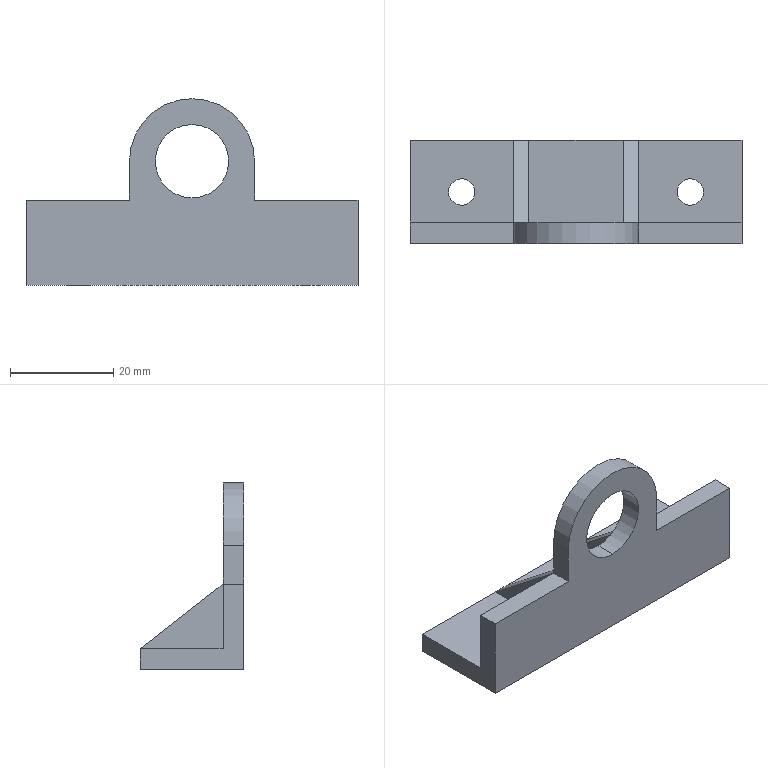Part | STEP file | Lead screw bearing sleeve | 1 solid | 28 faces | box 64.2 x 20 x 36.1 mm | volume 9790 mm3 | plane 21 | cylinder 7 | commonest cylinder face diameters 5.1 x4 14.2 x2 24.2 x1